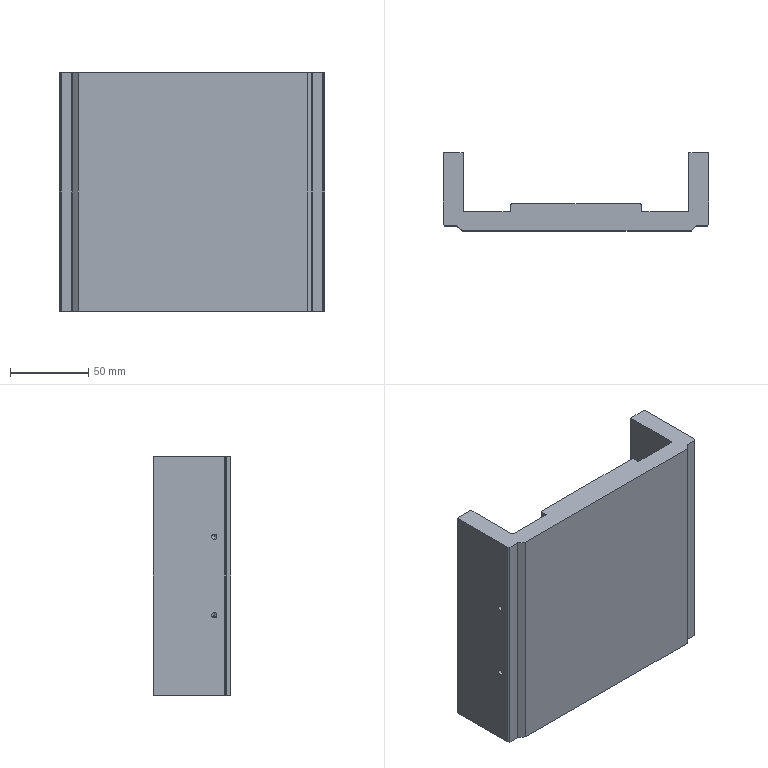Part | STEP file | 复件 FHB175-004^FHB175S-PRW-P40(马达RightUpper折-400W伺服电机) | 1 solid | 88 faces | box 169 x 49.5 x 152 mm | volume 495941 mm3 | cylinder 40 | cone 28 | plane 20 | commonest cylinder face diameters 6.8 x16 1 x10 3.3 x8 6 x4 3 x2